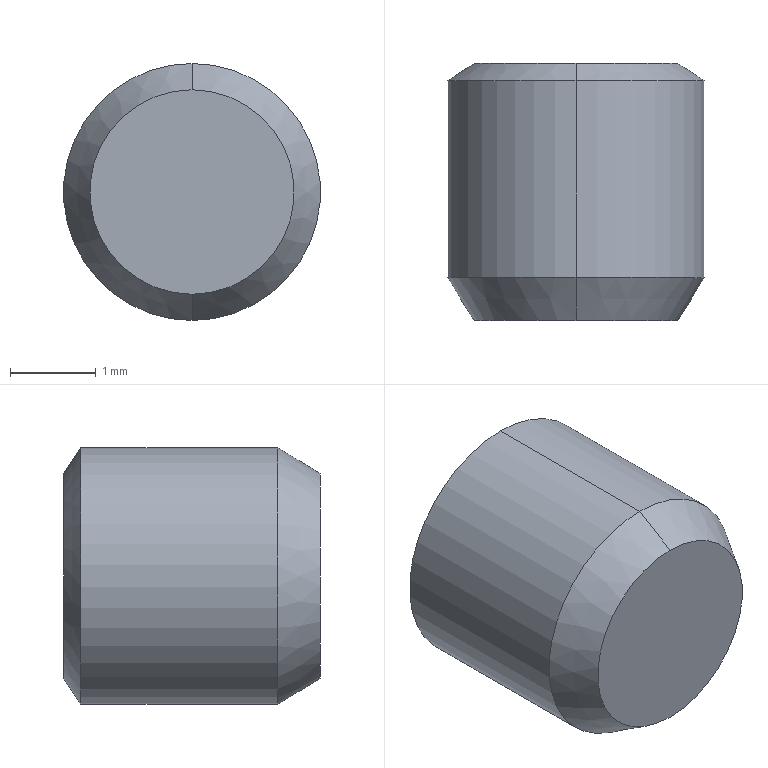Part | SolidWorks | features BaseBody 1 | 1 solid | 15 faces | box 3 x 3 x 3 mm | volume 17.925 mm3 | plane 9 | cone 4 | cylinder 2 | commonest cylinder face diameters 3 x2
STEP:
#1=CARTESIAN_POINT('',(0.,0.5,1.5));
#2=VERTEX_POINT('',#1);
#3=CARTESIAN_POINT('',(0.,0.5,-1.5));
#4=VERTEX_POINT('',#3);
#5=CARTESIAN_POINT('',(0.,0.5,0.));
#6=DIRECTION('',(0.,1.,0.));
#7=DIRECTION('',(0.,0.,1.));
#8=AXIS2_PLACEMENT_3D('',#5,#6,#7);
#9=CIRCLE('',#8,1.5);
#10=EDGE_CURVE('',#2,#4,#9,.T.);
#11=ORIENTED_EDGE('',*,*,#10,.T.);
#12=CARTESIAN_POINT('',(0.,2.8,-1.5));
#13=VERTEX_POINT('',#12);
#14=CARTESIAN_POINT('',(0.,0.,-1.5));
#15=DIRECTION('',(0.,1.,0.));
#16=VECTOR('',#15,1000.);
#17=LINE('',#14,#16);
#18=EDGE_CURVE('',#4,#13,#17,.T.);
#19=ORIENTED_EDGE('',*,*,#18,.T.);
#20=CARTESIAN_POINT('',(0.,2.8,1.5));
#21=VERTEX_POINT('',#20);
#22=CARTESIAN_POINT('',(0.,2.8,0.));
#23=DIRECTION('',(0.,-1.,0.));
#24=DIRECTION('',(0.,0.,1.));
#25=AXIS2_PLACEMENT_3D('',#22,#23,#24);
#26=CIRCLE('',#25,1.5);
#27=EDGE_CURVE('',#13,#21,#26,.T.);
#28=ORIENTED_EDGE('',*,*,#27,.T.);
#29=CARTESIAN_POINT('',(0.,0.,1.5));
#30=DIRECTION('',(0.,1.,0.));
#31=VECTOR('',#30,1000.);
#32=LINE('',#29,#31);
#33=EDGE_CURVE('',#2,#21,#32,.T.);
#34=ORIENTED_EDGE('',*,*,#33,.F.);
#35=EDGE_LOOP('',(#11,#19,#28,#34));
#36=FACE_OUTER_BOUND('',#35,.T.);
#37=CARTESIAN_POINT('',(0.,0.,0.));
#38=DIRECTION('',(0.,1.,0.));
#39=DIRECTION('',(0.,0.,1.));
#40=AXIS2_PLACEMENT_3D('',#37,#38,#39);
#41=CYLINDRICAL_SURFACE('',#40,1.5);
#42=ADVANCED_FACE('',(#36),#41,.T.);
#43=CARTESIAN_POINT('',(0.,3.,-1.193));
#44=VERTEX_POINT('',#43);
#45=CARTESIAN_POINT('',(0.,3.,1.193));
#46=VERTEX_POINT('',#45);
#47=CARTESIAN_POINT('',(0.,3.,0.));
#48=DIRECTION('',(0.,-1.,0.));
#49=DIRECTION('',(0.,0.,-1.));
#50=AXIS2_PLACEMENT_3D('',#47,#48,#49);
#51=CIRCLE('',#50,1.193);
#52=EDGE_CURVE('',#44,#46,#51,.T.);
#53=ORIENTED_EDGE('',*,*,#52,.T.);
#54=CARTESIAN_POINT('',(0.,2.8,1.5));
#55=DIRECTION('',(0.,-0.5465,0.8375));
#56=VECTOR('',#55,1000.);
#57=LINE('',#54,#56);
#58=EDGE_CURVE('',#46,#21,#57,.T.);
#59=ORIENTED_EDGE('',*,*,#58,.T.);
#60=ORIENTED_EDGE('',*,*,#27,.F.);
#61=CARTESIAN_POINT('',(0.,2.8,-1.5));
#62=DIRECTION('',(0.,-0.5465,-0.8375));
#63=VECTOR('',#62,1000.);
#64=LINE('',#61,#63);
#65=EDGE_CURVE('',#44,#13,#64,.T.);
#66=ORIENTED_EDGE('',*,*,#65,.F.);
#67=EDGE_LOOP('',(#53,#59,#60,#66));
#68=FACE_OUTER_BOUND('',#67,.T.);
#69=CARTESIAN_POINT('',(0.,2.8,0.));
#70=DIRECTION('',(0.,-1.,0.));
#71=DIRECTION('',(0.,0.,-1.));
#72=AXIS2_PLACEMENT_3D('',#69,#70,#71);
#73=CONICAL_SURFACE('',#72,1.5,0.9926);
#74=ADVANCED_FACE('',(#68),#73,.T.);
#75=CARTESIAN_POINT('',(0.,0.,1.194));
#76=VERTEX_POINT('',#75);
#77=CARTESIAN_POINT('',(0.,0.,-1.194));
#78=VERTEX_POINT('',#77);
#79=CARTESIAN_POINT('',(0.,0.,0.));
#80=DIRECTION('',(0.,1.,0.));
#81=DIRECTION('',(0.,0.,1.));
#82=AXIS2_PLACEMENT_3D('',#79,#80,#81);
#83=CIRCLE('',#82,1.194);
#84=EDGE_CURVE('',#76,#78,#83,.T.);
#85=ORIENTED_EDGE('',*,*,#84,.T.);
#86=CARTESIAN_POINT('',(0.,0.5,-1.5));
#87=DIRECTION('',(0.,0.8526,-0.5226));
#88=VECTOR('',#87,1000.);
#89=LINE('',#86,#88);
#90=EDGE_CURVE('',#78,#4,#89,.T.);
#91=ORIENTED_EDGE('',*,*,#90,.T.);
#92=ORIENTED_EDGE('',*,*,#10,.F.);
#93=CARTESIAN_POINT('',(0.,0.5,1.5));
#94=DIRECTION('',(0.,0.8526,0.5226));
#95=VECTOR('',#94,1000.);
#96=LINE('',#93,#95);
#97=EDGE_CURVE('',#76,#2,#96,.T.);
#98=ORIENTED_EDGE('',*,*,#97,.F.);
#99=EDGE_LOOP('',(#85,#91,#92,#98));
#100=FACE_OUTER_BOUND('',#99,.T.);
#101=CARTESIAN_POINT('',(0.,0.5,0.));
#102=DIRECTION('',(0.,1.,0.));
#103=DIRECTION('',(0.,0.,1.));
#104=AXIS2_PLACEMENT_3D('',#101,#102,#103);
#105=CONICAL_SURFACE('',#104,1.5,0.5499);
#106=ADVANCED_FACE('',(#100),#105,.T.);
#107=ORIENTED_EDGE('',*,*,#18,.F.);
#108=CARTESIAN_POINT('',(0.,0.5,0.));
#109=DIRECTION('',(0.,1.,0.));
#110=DIRECTION('',(0.,0.,1.));
#111=AXIS2_PLACEMENT_3D('',#108,#109,#110);
#112=CIRCLE('',#111,1.5);
#113=EDGE_CURVE('',#4,#2,#112,.T.);
#114=ORIENTED_EDGE('',*,*,#113,.T.);
#115=ORIENTED_EDGE('',*,*,#33,.T.);
#116=CARTESIAN_POINT('',(0.,2.8,0.));
#117=DIRECTION('',(0.,-1.,0.));
#118=DIRECTION('',(0.,0.,1.));
#119=AXIS2_PLACEMENT_3D('',#116,#117,#118);
#120=CIRCLE('',#119,1.5);
#121=EDGE_CURVE('',#21,#13,#120,.T.);
#122=ORIENTED_EDGE('',*,*,#121,.T.);
#123=EDGE_LOOP('',(#107,#114,#115,#122));
#124=FACE_OUTER_BOUND('',#123,.T.);
#125=CARTESIAN_POINT('',(0.,0.,0.));
#126=DIRECTION('',(0.,1.,0.));
#127=DIRECTION('',(0.,0.,1.));
#128=AXIS2_PLACEMENT_3D('',#125,#126,#127);
#129=CYLINDRICAL_SURFACE('',#128,1.5);
#130=ADVANCED_FACE('',(#124),#129,.T.);
#131=ORIENTED_EDGE('',*,*,#58,.F.);
#132=CARTESIAN_POINT('',(0.,3.,0.));
#133=DIRECTION('',(0.,-1.,0.));
#134=DIRECTION('',(0.,0.,-1.));
#135=AXIS2_PLACEMENT_3D('',#132,#133,#134);
#136=CIRCLE('',#135,1.193);
#137=EDGE_CURVE('',#46,#44,#136,.T.);
#138=ORIENTED_EDGE('',*,*,#137,.T.);
#139=ORIENTED_EDGE('',*,*,#65,.T.);
#140=ORIENTED_EDGE('',*,*,#121,.F.);
#141=EDGE_LOOP('',(#131,#138,#139,#140));
#142=FACE_OUTER_BOUND('',#141,.T.);
#143=CARTESIAN_POINT('',(0.,2.8,0.));
#144=DIRECTION('',(0.,-1.,0.));
#145=DIRECTION('',(0.,0.,-1.));
#146=AXIS2_PLACEMENT_3D('',#143,#144,#145);
#147=CONICAL_SURFACE('',#146,1.5,0.9926);
#148=ADVANCED_FACE('',(#142),#147,.T.);
#149=ORIENTED_EDGE('',*,*,#90,.F.);
#150=CARTESIAN_POINT('',(0.,0.,0.));
#151=DIRECTION('',(0.,1.,0.));
#152=DIRECTION('',(0.,0.,1.));
#153=AXIS2_PLACEMENT_3D('',#150,#151,#152);
#154=CIRCLE('',#153,1.194);
#155=EDGE_CURVE('',#78,#76,#154,.T.);
#156=ORIENTED_EDGE('',*,*,#155,.T.);
#157=ORIENTED_EDGE('',*,*,#97,.T.);
#158=ORIENTED_EDGE('',*,*,#113,.F.);
#159=EDGE_LOOP('',(#149,#156,#157,#158));
#160=FACE_OUTER_BOUND('',#159,.T.);
#161=CARTESIAN_POINT('',(0.,0.5,0.));
#162=DIRECTION('',(0.,1.,0.));
#163=DIRECTION('',(0.,0.,1.));
#164=AXIS2_PLACEMENT_3D('',#161,#162,#163);
#165=CONICAL_SURFACE('',#164,1.5,0.5499);
#166=ADVANCED_FACE('',(#160),#165,.T.);
#167=CARTESIAN_POINT('',(-0.75,3.,0.433));
#168=VERTEX_POINT('',#167);
#169=CARTESIAN_POINT('',(0.,3.,0.866));
#170=VERTEX_POINT('',#169);
#171=CARTESIAN_POINT('',(-0.75,3.,0.433));
#172=DIRECTION('',(0.866,0.,0.5));
#173=VECTOR('',#172,1000.);
#174=LINE('',#171,#173);
#175=EDGE_CURVE('',#168,#170,#174,.T.);
#176=ORIENTED_EDGE('',*,*,#175,.F.);
#177=CARTESIAN_POINT('',(-0.75,3.,-0.433));
#178=VERTEX_POINT('',#177);
#179=CARTESIAN_POINT('',(-0.75,3.,0.));
#180=DIRECTION('',(0.,0.,1.));
#181=VECTOR('',#180,1000.);
#182=LINE('',#179,#181);
#183=EDGE_CURVE('',#178,#168,#182,.T.);
#184=ORIENTED_EDGE('',*,*,#183,.F.);
#185=CARTESIAN_POINT('',(0.,3.,-0.866));
#186=VERTEX_POINT('',#185);
#187=CARTESIAN_POINT('',(0.,3.,-0.866));
#188=DIRECTION('',(-0.866,0.,0.5));
#189=VECTOR('',#188,1000.);
#190=LINE('',#187,#189);
#191=EDGE_CURVE('',#186,#178,#190,.T.);
#192=ORIENTED_EDGE('',*,*,#191,.F.);
#193=CARTESIAN_POINT('',(0.75,3.,-0.433));
#194=VERTEX_POINT('',#193);
#195=CARTESIAN_POINT('',(0.75,3.,-0.433));
#196=DIRECTION('',(-0.866,0.,-0.5));
#197=VECTOR('',#196,1000.);
#198=LINE('',#195,#197);
#199=EDGE_CURVE('',#194,#186,#198,.T.);
#200=ORIENTED_EDGE('',*,*,#199,.F.);
#201=CARTESIAN_POINT('',(0.75,3.,0.433));
#202=VERTEX_POINT('',#201);
#203=CARTESIAN_POINT('',(0.75,3.,0.));
#204=DIRECTION('',(0.,0.,-1.));
#205=VECTOR('',#204,1000.);
#206=LINE('',#203,#205);
#207=EDGE_CURVE('',#202,#194,#206,.T.);
#208=ORIENTED_EDGE('',*,*,#207,.F.);
#209=CARTESIAN_POINT('',(0.,3.,0.866));
#210=DIRECTION('',(0.866,0.,-0.5));
#211=VECTOR('',#210,1000.);
#212=LINE('',#209,#211);
#213=EDGE_CURVE('',#170,#202,#212,.T.);
#214=ORIENTED_EDGE('',*,*,#213,.F.);
#215=EDGE_LOOP('',(#176,#184,#192,#200,#208,#214));
#216=FACE_BOUND('',#215,.T.);
#217=ORIENTED_EDGE('',*,*,#52,.F.);
#218=ORIENTED_EDGE('',*,*,#137,.F.);
#219=EDGE_LOOP('',(#217,#218));
#220=FACE_OUTER_BOUND('',#219,.T.);
#221=CARTESIAN_POINT('',(0.,3.,0.));
#222=DIRECTION('',(0.,-1.,0.));
#223=DIRECTION('',(0.,0.,-1.));
#224=AXIS2_PLACEMENT_3D('',#221,#222,#223);
#225=PLANE('',#224);
#226=ADVANCED_FACE('',(#216,#220),#225,.F.);
#227=ORIENTED_EDGE('',*,*,#84,.F.);
#228=ORIENTED_EDGE('',*,*,#155,.F.);
#229=EDGE_LOOP('',(#227,#228));
#230=FACE_OUTER_BOUND('',#229,.T.);
#231=CARTESIAN_POINT('',(1.194,0.,0.));
#232=DIRECTION('',(0.,1.,0.));
#233=DIRECTION('',(0.,0.,1.));
#234=AXIS2_PLACEMENT_3D('',#231,#232,#233);
#235=PLANE('',#234);
#236=ADVANCED_FACE('',(#230),#235,.F.);
#237=CARTESIAN_POINT('',(0.75,1.8,0.433));
#238=VERTEX_POINT('',#237);
#239=CARTESIAN_POINT('',(0.75,1.8,0.433));
#240=DIRECTION('',(0.,1.,0.));
#241=VECTOR('',#240,1000.);
#242=LINE('',#239,#241);
#243=EDGE_CURVE('',#238,#202,#242,.T.);
#244=ORIENTED_EDGE('',*,*,#243,.F.);
#245=CARTESIAN_POINT('',(0.,1.8,0.866));
#246=VERTEX_POINT('',#245);
#247=CARTESIAN_POINT('',(0.,1.8,0.866));
#248=DIRECTION('',(0.866,0.,-0.5));
#249=VECTOR('',#248,1000.);
#250=LINE('',#247,#249);
#251=EDGE_CURVE('',#246,#238,#250,.T.);
#252=ORIENTED_EDGE('',*,*,#251,.F.);
#253=CARTESIAN_POINT('',(0.,1.8,0.866));
#254=DIRECTION('',(0.,-1.,0.));
#255=VECTOR('',#254,1000.);
#256=LINE('',#253,#255);
#257=EDGE_CURVE('',#170,#246,#256,.T.);
#258=ORIENTED_EDGE('',*,*,#257,.F.);
#259=ORIENTED_EDGE('',*,*,#213,.T.);
#260=EDGE_LOOP('',(#244,#252,#258,#259));
#261=FACE_OUTER_BOUND('',#260,.T.);
#262=CARTESIAN_POINT('',(0.,1.8,0.866));
#263=DIRECTION('',(0.5,0.,0.866));
#264=DIRECTION('',(0.866,0.,-0.5));
#265=AXIS2_PLACEMENT_3D('',#262,#263,#264);
#266=PLANE('',#265);
#267=ADVANCED_FACE('',(#261),#266,.F.);
#268=ORIENTED_EDGE('',*,*,#257,.T.);
#269=CARTESIAN_POINT('',(-0.75,1.8,0.433));
#270=VERTEX_POINT('',#269);
#271=CARTESIAN_POINT('',(-0.75,1.8,0.433));
#272=DIRECTION('',(0.866,0.,0.5));
#273=VECTOR('',#272,1000.);
#274=LINE('',#271,#273);
#275=EDGE_CURVE('',#270,#246,#274,.T.);
#276=ORIENTED_EDGE('',*,*,#275,.F.);
#277=CARTESIAN_POINT('',(-0.75,1.8,0.433));
#278=DIRECTION('',(0.,-1.,0.));
#279=VECTOR('',#278,1000.);
#280=LINE('',#277,#279);
#281=EDGE_CURVE('',#168,#270,#280,.T.);
#282=ORIENTED_EDGE('',*,*,#281,.F.);
#283=ORIENTED_EDGE('',*,*,#175,.T.);
#284=EDGE_LOOP('',(#268,#276,#282,#283));
#285=FACE_OUTER_BOUND('',#284,.T.);
#286=CARTESIAN_POINT('',(-0.75,1.8,0.433));
#287=DIRECTION('',(-0.5,0.,0.866));
#288=DIRECTION('',(0.866,0.,0.5));
#289=AXIS2_PLACEMENT_3D('',#286,#287,#288);
#290=PLANE('',#289);
#291=ADVANCED_FACE('',(#285),#290,.F.);
#292=ORIENTED_EDGE('',*,*,#281,.T.);
#293=CARTESIAN_POINT('',(-0.75,1.8,-0.433));
#294=VERTEX_POINT('',#293);
#295=CARTESIAN_POINT('',(-0.75,1.8,-0.433));
#296=DIRECTION('',(0.,0.,1.));
#297=VECTOR('',#296,1000.);
#298=LINE('',#295,#297);
#299=EDGE_CURVE('',#294,#270,#298,.T.);
#300=ORIENTED_EDGE('',*,*,#299,.F.);
#301=CARTESIAN_POINT('',(-0.75,1.8,-0.433));
#302=DIRECTION('',(0.,-1.,0.));
#303=VECTOR('',#302,1000.);
#304=LINE('',#301,#303);
#305=EDGE_CURVE('',#178,#294,#304,.T.);
#306=ORIENTED_EDGE('',*,*,#305,.F.);
#307=ORIENTED_EDGE('',*,*,#183,.T.);
#308=EDGE_LOOP('',(#292,#300,#306,#307));
#309=FACE_OUTER_BOUND('',#308,.T.);
#310=CARTESIAN_POINT('',(-0.75,1.8,-0.433));
#311=DIRECTION('',(-1.,0.,0.));
#312=DIRECTION('',(0.,0.,1.));
#313=AXIS2_PLACEMENT_3D('',#310,#311,#312);
#314=PLANE('',#313);
#315=ADVANCED_FACE('',(#309),#314,.F.);
#316=ORIENTED_EDGE('',*,*,#305,.T.);
#317=CARTESIAN_POINT('',(0.,1.8,-0.866));
#318=VERTEX_POINT('',#317);
#319=CARTESIAN_POINT('',(0.,1.8,-0.866));
#320=DIRECTION('',(-0.866,0.,0.5));
#321=VECTOR('',#320,1000.);
#322=LINE('',#319,#321);
#323=EDGE_CURVE('',#318,#294,#322,.T.);
#324=ORIENTED_EDGE('',*,*,#323,.F.);
#325=CARTESIAN_POINT('',(0.,1.8,-0.866));
#326=DIRECTION('',(0.,-1.,0.));
#327=VECTOR('',#326,1000.);
#328=LINE('',#325,#327);
#329=EDGE_CURVE('',#186,#318,#328,.T.);
#330=ORIENTED_EDGE('',*,*,#329,.F.);
#331=ORIENTED_EDGE('',*,*,#191,.T.);
#332=EDGE_LOOP('',(#316,#324,#330,#331));
#333=FACE_OUTER_BOUND('',#332,.T.);
#334=CARTESIAN_POINT('',(0.,1.8,-0.866));
#335=DIRECTION('',(-0.5,0.,-0.866));
#336=DIRECTION('',(-0.866,0.,0.5));
#337=AXIS2_PLACEMENT_3D('',#334,#335,#336);
#338=PLANE('',#337);
#339=ADVANCED_FACE('',(#333),#338,.F.);
#340=ORIENTED_EDGE('',*,*,#329,.T.);
#341=CARTESIAN_POINT('',(0.75,1.8,-0.433));
#342=VERTEX_POINT('',#341);
#343=CARTESIAN_POINT('',(0.75,1.8,-0.433));
#344=DIRECTION('',(-0.866,0.,-0.5));
#345=VECTOR('',#344,1000.);
#346=LINE('',#343,#345);
#347=EDGE_CURVE('',#342,#318,#346,.T.);
#348=ORIENTED_EDGE('',*,*,#347,.F.);
#349=CARTESIAN_POINT('',(0.75,1.8,-0.433));
#350=DIRECTION('',(0.,-1.,0.));
#351=VECTOR('',#350,1000.);
#352=LINE('',#349,#351);
#353=EDGE_CURVE('',#194,#342,#352,.T.);
#354=ORIENTED_EDGE('',*,*,#353,.F.);
#355=ORIENTED_EDGE('',*,*,#199,.T.);
#356=EDGE_LOOP('',(#340,#348,#354,#355));
#357=FACE_OUTER_BOUND('',#356,.T.);
#358=CARTESIAN_POINT('',(0.75,1.8,-0.433));
#359=DIRECTION('',(0.5,0.,-0.866));
#360=DIRECTION('',(-0.866,0.,-0.5));
#361=AXIS2_PLACEMENT_3D('',#358,#359,#360);
#362=PLANE('',#361);
#363=ADVANCED_FACE('',(#357),#362,.F.);
#364=ORIENTED_EDGE('',*,*,#207,.T.);
#365=ORIENTED_EDGE('',*,*,#353,.T.);
#366=CARTESIAN_POINT('',(0.75,1.8,0.433));
#367=DIRECTION('',(0.,0.,-1.));
#368=VECTOR('',#367,1000.);
#369=LINE('',#366,#368);
#370=EDGE_CURVE('',#238,#342,#369,.T.);
#371=ORIENTED_EDGE('',*,*,#370,.F.);
#372=ORIENTED_EDGE('',*,*,#243,.T.);
#373=EDGE_LOOP('',(#364,#365,#371,#372));
#374=FACE_OUTER_BOUND('',#373,.T.);
#375=CARTESIAN_POINT('',(0.75,1.8,0.433));
#376=DIRECTION('',(1.,0.,0.));
#377=DIRECTION('',(0.,0.,-1.));
#378=AXIS2_PLACEMENT_3D('',#375,#376,#377);
#379=PLANE('',#378);
#380=ADVANCED_FACE('',(#374),#379,.F.);
#381=ORIENTED_EDGE('',*,*,#347,.T.);
#382=ORIENTED_EDGE('',*,*,#323,.T.);
#383=ORIENTED_EDGE('',*,*,#299,.T.);
#384=ORIENTED_EDGE('',*,*,#275,.T.);
#385=ORIENTED_EDGE('',*,*,#251,.T.);
#386=ORIENTED_EDGE('',*,*,#370,.T.);
#387=EDGE_LOOP('',(#381,#382,#383,#384,#385,#386));
#388=FACE_OUTER_BOUND('',#387,.T.);
#389=CARTESIAN_POINT('',(0.,1.8,0.));
#390=DIRECTION('',(0.,1.,0.));
#391=DIRECTION('',(0.,0.,1.));
#392=AXIS2_PLACEMENT_3D('',#389,#390,#391);
#393=PLANE('',#392);
#394=ADVANCED_FACE('',(#388),#393,.T.);
#395=CLOSED_SHELL('',(#42,#74,#106,#130,#148,#166,#226,#236,#267,#291,#315,#339,#363,#380,#394));
#396=MANIFOLD_SOLID_BREP('',#395);
#397=CARTESIAN_POINT('',(0.,0.,0.));
#398=DIRECTION('',(0.,0.,1.));
#399=DIRECTION('',(1.,0.,0.));
#400=AXIS2_PLACEMENT_3D('',#397,#398,#399);
#401=(LENGTH_UNIT()NAMED_UNIT(*)SI_UNIT(.MILLI.,.METRE.));
#402=UNCERTAINTY_MEASURE_WITH_UNIT(LENGTH_MEASURE(0.00001),#401,'','');
#403=(NAMED_UNIT(*)PLANE_ANGLE_UNIT()SI_UNIT($,.RADIAN.));
#404=(NAMED_UNIT(*)SI_UNIT($,.STERADIAN.)SOLID_ANGLE_UNIT());
#405=(GEOMETRIC_REPRESENTATION_CONTEXT(3)GLOBAL_UNCERTAINTY_ASSIGNED_CONTEXT((#402))GLOBAL_UNIT_ASSIGNED_CONTEXT((#401,#403,#404))REPRESENTATION_CONTEXT('',''));
#406=ADVANCED_BREP_SHAPE_REPRESENTATION('',(#396,#400),#405);